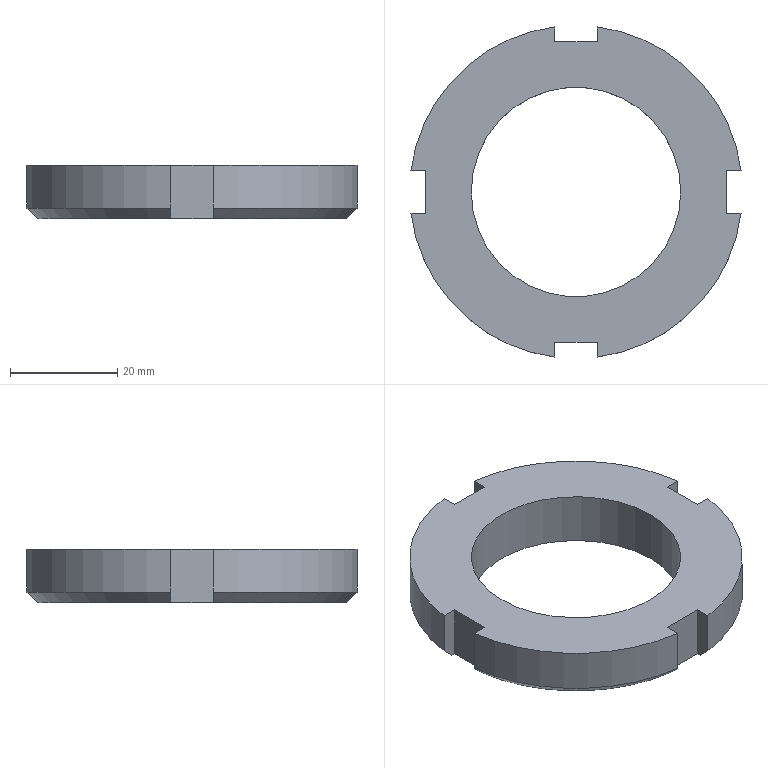Part | STEP file | M42 nut | 1 solid | 24 faces | box 61.482 x 61.482 x 10 mm | volume 16995 mm3 | plane 14 | cylinder 6 | cone 4 | commonest cylinder face diameters 62 x4 39 x2